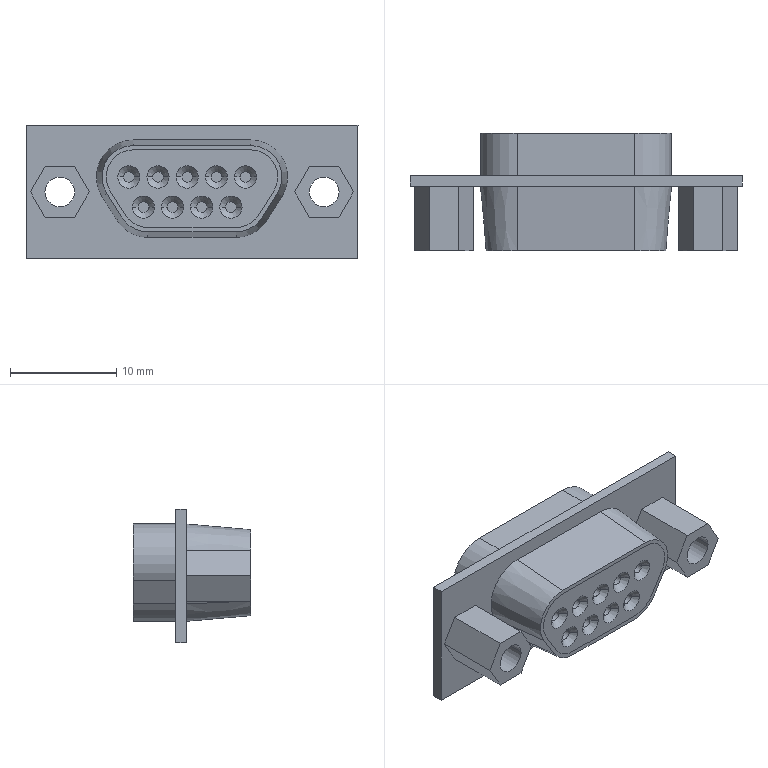Part | NX | features BREP 1 | 1 solid | 97 faces | box 31.31 x 11.07 x 12.55 mm | volume 1882 mm3 | plane 44 | cylinder 31 | cone 22 | commonest cylinder face diameters 1 x18 5.098 x5 2.8 x4 6.96 x4